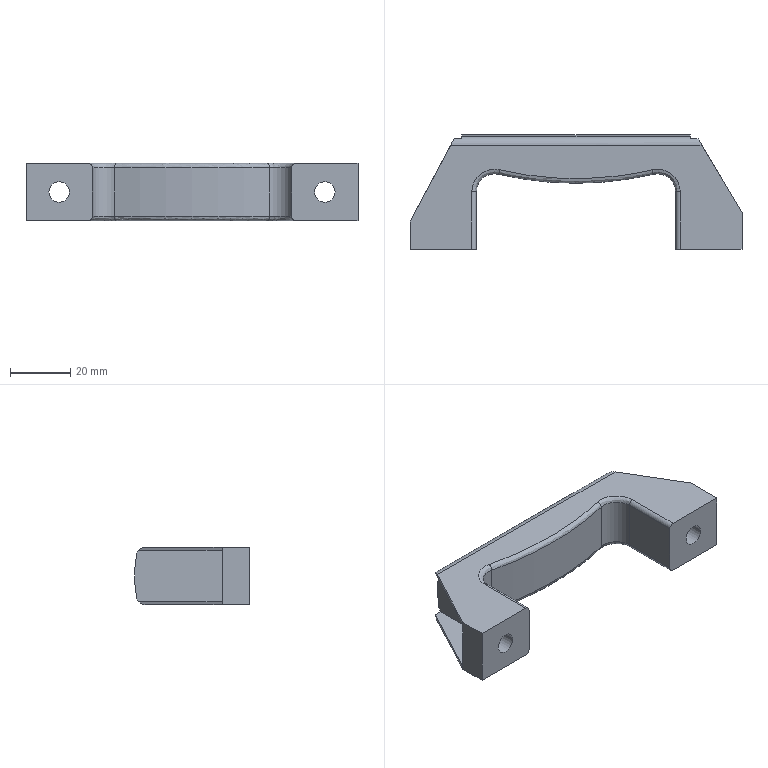Part | SolidWorks | features BaseBody 1 | 1 solid | 46 faces | box 110 x 38 x 19 mm | volume 30744 mm3 | plane 22 | cylinder 18 | spline 6 | commonest cylinder face diameters 3 x4 6.8 x4 10.88 x4 6 x2 12 x2 76 x1